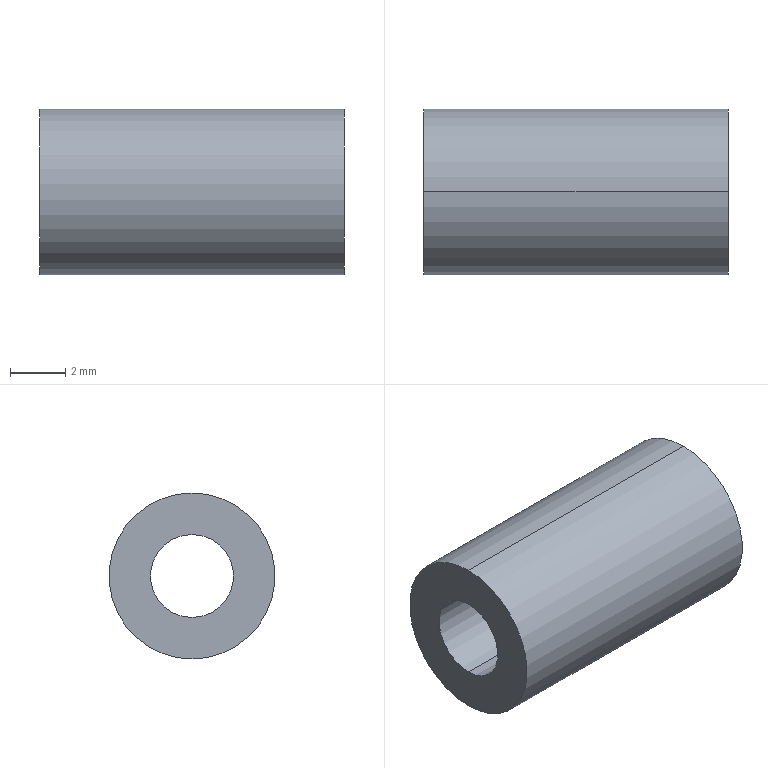Part | STEP file | Stud_1 | 1 solid | 6 faces | box 11 x 6 x 6 mm | volume 233.263 mm3 | cylinder 4 | plane 2 | commonest cylinder face diameters 3 x2 6 x2
STEP:
#1=CARTESIAN_POINT('',(0.,0.,0.));
#2=DIRECTION('',(0.,0.,1.));
#3=DIRECTION('',(1.,0.,0.));
#4=AXIS2_PLACEMENT_3D('',#1,#2,#3);
#5=CARTESIAN_POINT('',(11.,0.,3.));
#6=VERTEX_POINT('',#5);
#7=CARTESIAN_POINT('',(11.,0.,-3.));
#8=VERTEX_POINT('',#7);
#9=CARTESIAN_POINT('',(11.,0.,0.));
#10=DIRECTION('',(-1.,0.,0.));
#11=DIRECTION('',(0.,0.,1.));
#12=AXIS2_PLACEMENT_3D('',#9,#10,#11);
#13=CIRCLE('',#12,3.);
#14=CARTESIAN_POINT('',(11.,0.,0.));
#15=DIRECTION('',(-1.,0.,0.));
#16=DIRECTION('',(0.,0.,1.));
#17=AXIS2_PLACEMENT_3D('',#14,#15,#16);
#18=CYLINDRICAL_SURFACE('',#17,3.);
#19=CARTESIAN_POINT('',(0.,0.));
#20=DIRECTION('',(1.,0.));
#21=VECTOR('',#20,1.);
#22=LINE('',#19,#21);
#23=(GEOMETRIC_REPRESENTATION_CONTEXT(2)PARAMETRIC_REPRESENTATION_CONTEXT()REPRESENTATION_CONTEXT('',''));
#24=DEFINITIONAL_REPRESENTATION('',(#22),#23);
#25=PCURVE('',#18,#24);
#26=CARTESIAN_POINT('',(11.,0.,0.));
#27=DIRECTION('',(1.,0.,0.));
#28=DIRECTION('',(0.,0.,-1.));
#29=AXIS2_PLACEMENT_3D('',#26,#27,#28);
#30=PLANE('',#29);
#31=CARTESIAN_POINT('',(-3.,0.));
#32=CARTESIAN_POINT('',(-3.,5.196));
#33=CARTESIAN_POINT('',(1.5,2.598));
#34=CARTESIAN_POINT('',(6.,0.));
#35=CARTESIAN_POINT('',(1.5,-2.598));
#36=CARTESIAN_POINT('',(-3.,-5.196));
#37=CARTESIAN_POINT('',(-3.,0.));
#38=(BOUNDED_CURVE()B_SPLINE_CURVE(2,(#31,#32,#33,#34,#35,#36,#37),.UNSPECIFIED.,.T.,.F.)B_SPLINE_CURVE_WITH_KNOTS((1,2,2,2,2,1),(-2.094,0.,2.094,4.189,6.283,8.378),.UNSPECIFIED.)CURVE()GEOMETRIC_REPRESENTATION_ITEM()RATIONAL_B_SPLINE_CURVE((1.,0.5,1.,0.5,1.,0.5,1.))REPRESENTATION_ITEM(''));
#39=(GEOMETRIC_REPRESENTATION_CONTEXT(2)PARAMETRIC_REPRESENTATION_CONTEXT()REPRESENTATION_CONTEXT('',''));
#40=DEFINITIONAL_REPRESENTATION('',(#38),#39);
#41=PCURVE('',#30,#40);
#42=SURFACE_CURVE('',#13,(#25,#41),.PCURVE_S1.);
#43=EDGE_CURVE('',#6,#8,#42,.T.);
#44=ORIENTED_EDGE('',*,*,#43,.T.);
#45=CARTESIAN_POINT('',(0.,0.,-3.));
#46=VERTEX_POINT('',#45);
#47=CARTESIAN_POINT('',(11.,0.,-3.));
#48=DIRECTION('',(-1.,0.,0.));
#49=VECTOR('',#48,1.);
#50=LINE('',#47,#49);
#51=CARTESIAN_POINT('',(3.142,0.));
#52=DIRECTION('',(0.,1.));
#53=VECTOR('',#52,1.);
#54=LINE('',#51,#53);
#55=(GEOMETRIC_REPRESENTATION_CONTEXT(2)PARAMETRIC_REPRESENTATION_CONTEXT()REPRESENTATION_CONTEXT('',''));
#56=DEFINITIONAL_REPRESENTATION('',(#54),#55);
#57=PCURVE('',#18,#56);
#58=CARTESIAN_POINT('',(11.,0.,0.));
#59=DIRECTION('',(-1.,0.,0.));
#60=DIRECTION('',(0.,0.,1.));
#61=AXIS2_PLACEMENT_3D('',#58,#59,#60);
#62=CYLINDRICAL_SURFACE('',#61,3.);
#63=CARTESIAN_POINT('',(3.142,0.));
#64=DIRECTION('',(0.,1.));
#65=VECTOR('',#64,1.);
#66=LINE('',#63,#65);
#67=(GEOMETRIC_REPRESENTATION_CONTEXT(2)PARAMETRIC_REPRESENTATION_CONTEXT()REPRESENTATION_CONTEXT('',''));
#68=DEFINITIONAL_REPRESENTATION('',(#66),#67);
#69=PCURVE('',#62,#68);
#70=SURFACE_CURVE('',#50,(#57,#69),.PCURVE_S1.);
#71=EDGE_CURVE('',#8,#46,#70,.T.);
#72=ORIENTED_EDGE('',*,*,#71,.T.);
#73=CARTESIAN_POINT('',(0.,0.,3.));
#74=VERTEX_POINT('',#73);
#75=CARTESIAN_POINT('',(0.,0.,0.));
#76=DIRECTION('',(1.,0.,0.));
#77=DIRECTION('',(0.,0.,1.));
#78=AXIS2_PLACEMENT_3D('',#75,#76,#77);
#79=CIRCLE('',#78,3.);
#80=CARTESIAN_POINT('',(6.283,11.));
#81=DIRECTION('',(-1.,0.));
#82=VECTOR('',#81,1.);
#83=LINE('',#80,#82);
#84=(GEOMETRIC_REPRESENTATION_CONTEXT(2)PARAMETRIC_REPRESENTATION_CONTEXT()REPRESENTATION_CONTEXT('',''));
#85=DEFINITIONAL_REPRESENTATION('',(#83),#84);
#86=PCURVE('',#18,#85);
#87=CARTESIAN_POINT('',(0.,0.,0.));
#88=DIRECTION('',(1.,0.,0.));
#89=DIRECTION('',(0.,0.,-1.));
#90=AXIS2_PLACEMENT_3D('',#87,#88,#89);
#91=PLANE('',#90);
#92=CARTESIAN_POINT('',(0.,0.));
#93=DIRECTION('',(-1.,0.));
#94=AXIS2_PLACEMENT_2D('',#92,#93);
#95=CIRCLE('',#94,3.);
#96=(GEOMETRIC_REPRESENTATION_CONTEXT(2)PARAMETRIC_REPRESENTATION_CONTEXT()REPRESENTATION_CONTEXT('',''));
#97=DEFINITIONAL_REPRESENTATION('',(#95),#96);
#98=PCURVE('',#91,#97);
#99=SURFACE_CURVE('',#79,(#86,#98),.PCURVE_S1.);
#100=EDGE_CURVE('',#46,#74,#99,.T.);
#101=ORIENTED_EDGE('',*,*,#100,.T.);
#102=CARTESIAN_POINT('',(11.,0.,3.));
#103=DIRECTION('',(-1.,0.,0.));
#104=VECTOR('',#103,1.);
#105=LINE('',#102,#104);
#106=CARTESIAN_POINT('',(0.,0.));
#107=DIRECTION('',(0.,1.));
#108=VECTOR('',#107,1.);
#109=LINE('',#106,#108);
#110=(GEOMETRIC_REPRESENTATION_CONTEXT(2)PARAMETRIC_REPRESENTATION_CONTEXT()REPRESENTATION_CONTEXT('',''));
#111=DEFINITIONAL_REPRESENTATION('',(#109),#110);
#112=PCURVE('',#18,#111);
#113=CARTESIAN_POINT('',(6.283,0.));
#114=DIRECTION('',(0.,1.));
#115=VECTOR('',#114,1.);
#116=LINE('',#113,#115);
#117=(GEOMETRIC_REPRESENTATION_CONTEXT(2)PARAMETRIC_REPRESENTATION_CONTEXT()REPRESENTATION_CONTEXT('',''));
#118=DEFINITIONAL_REPRESENTATION('',(#116),#117);
#119=PCURVE('',#62,#118);
#120=SURFACE_CURVE('',#105,(#112,#119),.PCURVE_S1.);
#121=EDGE_CURVE('',#6,#74,#120,.T.);
#122=ORIENTED_EDGE('',*,*,#121,.F.);
#123=EDGE_LOOP('',(#44,#72,#101,#122));
#124=FACE_BOUND('',#123,.T.);
#125=ADVANCED_FACE('',(#124),#18,.T.);
#126=CARTESIAN_POINT('',(11.,0.,1.5));
#127=VERTEX_POINT('',#126);
#128=CARTESIAN_POINT('',(0.,0.,1.5));
#129=VERTEX_POINT('',#128);
#130=CARTESIAN_POINT('',(11.,0.,1.5));
#131=DIRECTION('',(-1.,0.,0.));
#132=VECTOR('',#131,1.);
#133=LINE('',#130,#132);
#134=CARTESIAN_POINT('',(11.,0.,0.));
#135=DIRECTION('',(-1.,0.,0.));
#136=DIRECTION('',(0.,0.,1.));
#137=AXIS2_PLACEMENT_3D('',#134,#135,#136);
#138=CYLINDRICAL_SURFACE('',#137,1.5);
#139=CARTESIAN_POINT('',(6.283,0.));
#140=DIRECTION('',(0.,1.));
#141=VECTOR('',#140,1.);
#142=LINE('',#139,#141);
#143=(GEOMETRIC_REPRESENTATION_CONTEXT(2)PARAMETRIC_REPRESENTATION_CONTEXT()REPRESENTATION_CONTEXT('',''));
#144=DEFINITIONAL_REPRESENTATION('',(#142),#143);
#145=PCURVE('',#138,#144);
#146=CARTESIAN_POINT('',(11.,0.,0.));
#147=DIRECTION('',(-1.,0.,0.));
#148=DIRECTION('',(0.,0.,1.));
#149=AXIS2_PLACEMENT_3D('',#146,#147,#148);
#150=CYLINDRICAL_SURFACE('',#149,1.5);
#151=CARTESIAN_POINT('',(0.,0.));
#152=DIRECTION('',(0.,1.));
#153=VECTOR('',#152,1.);
#154=LINE('',#151,#153);
#155=(GEOMETRIC_REPRESENTATION_CONTEXT(2)PARAMETRIC_REPRESENTATION_CONTEXT()REPRESENTATION_CONTEXT('',''));
#156=DEFINITIONAL_REPRESENTATION('',(#154),#155);
#157=PCURVE('',#150,#156);
#158=SURFACE_CURVE('',#133,(#145,#157),.PCURVE_S1.);
#159=EDGE_CURVE('',#127,#129,#158,.T.);
#160=ORIENTED_EDGE('',*,*,#159,.T.);
#161=CARTESIAN_POINT('',(0.,0.,-1.5));
#162=VERTEX_POINT('',#161);
#163=CARTESIAN_POINT('',(0.,0.,0.));
#164=DIRECTION('',(-1.,0.,0.));
#165=DIRECTION('',(0.,0.,1.));
#166=AXIS2_PLACEMENT_3D('',#163,#164,#165);
#167=CIRCLE('',#166,1.5);
#168=CARTESIAN_POINT('',(0.,11.));
#169=DIRECTION('',(1.,0.));
#170=VECTOR('',#169,1.);
#171=LINE('',#168,#170);
#172=(GEOMETRIC_REPRESENTATION_CONTEXT(2)PARAMETRIC_REPRESENTATION_CONTEXT()REPRESENTATION_CONTEXT('',''));
#173=DEFINITIONAL_REPRESENTATION('',(#171),#172);
#174=PCURVE('',#138,#173);
#175=CARTESIAN_POINT('',(-1.5,0.));
#176=CARTESIAN_POINT('',(-1.5,2.598));
#177=CARTESIAN_POINT('',(0.75,1.299));
#178=CARTESIAN_POINT('',(3.,0.));
#179=CARTESIAN_POINT('',(0.75,-1.299));
#180=CARTESIAN_POINT('',(-1.5,-2.598));
#181=CARTESIAN_POINT('',(-1.5,0.));
#182=(BOUNDED_CURVE()B_SPLINE_CURVE(2,(#175,#176,#177,#178,#179,#180,#181),.UNSPECIFIED.,.T.,.F.)B_SPLINE_CURVE_WITH_KNOTS((1,2,2,2,2,1),(-2.094,0.,2.094,4.189,6.283,8.378),.UNSPECIFIED.)CURVE()GEOMETRIC_REPRESENTATION_ITEM()RATIONAL_B_SPLINE_CURVE((1.,0.5,1.,0.5,1.,0.5,1.))REPRESENTATION_ITEM(''));
#183=(GEOMETRIC_REPRESENTATION_CONTEXT(2)PARAMETRIC_REPRESENTATION_CONTEXT()REPRESENTATION_CONTEXT('',''));
#184=DEFINITIONAL_REPRESENTATION('',(#182),#183);
#185=PCURVE('',#91,#184);
#186=SURFACE_CURVE('',#167,(#174,#185),.PCURVE_S1.);
#187=EDGE_CURVE('',#162,#129,#186,.T.);
#188=ORIENTED_EDGE('',*,*,#187,.F.);
#189=CARTESIAN_POINT('',(11.,0.,-1.5));
#190=VERTEX_POINT('',#189);
#191=CARTESIAN_POINT('',(11.,0.,-1.5));
#192=DIRECTION('',(-1.,0.,0.));
#193=VECTOR('',#192,1.);
#194=LINE('',#191,#193);
#195=CARTESIAN_POINT('',(3.142,0.));
#196=DIRECTION('',(0.,1.));
#197=VECTOR('',#196,1.);
#198=LINE('',#195,#197);
#199=(GEOMETRIC_REPRESENTATION_CONTEXT(2)PARAMETRIC_REPRESENTATION_CONTEXT()REPRESENTATION_CONTEXT('',''));
#200=DEFINITIONAL_REPRESENTATION('',(#198),#199);
#201=PCURVE('',#138,#200);
#202=CARTESIAN_POINT('',(3.142,0.));
#203=DIRECTION('',(0.,1.));
#204=VECTOR('',#203,1.);
#205=LINE('',#202,#204);
#206=(GEOMETRIC_REPRESENTATION_CONTEXT(2)PARAMETRIC_REPRESENTATION_CONTEXT()REPRESENTATION_CONTEXT('',''));
#207=DEFINITIONAL_REPRESENTATION('',(#205),#206);
#208=PCURVE('',#150,#207);
#209=SURFACE_CURVE('',#194,(#201,#208),.PCURVE_S1.);
#210=EDGE_CURVE('',#190,#162,#209,.T.);
#211=ORIENTED_EDGE('',*,*,#210,.F.);
#212=CARTESIAN_POINT('',(11.,0.,0.));
#213=DIRECTION('',(-1.,0.,0.));
#214=DIRECTION('',(0.,0.,1.));
#215=AXIS2_PLACEMENT_3D('',#212,#213,#214);
#216=CIRCLE('',#215,1.5);
#217=CARTESIAN_POINT('',(0.,0.));
#218=DIRECTION('',(1.,0.));
#219=VECTOR('',#218,1.);
#220=LINE('',#217,#219);
#221=(GEOMETRIC_REPRESENTATION_CONTEXT(2)PARAMETRIC_REPRESENTATION_CONTEXT()REPRESENTATION_CONTEXT('',''));
#222=DEFINITIONAL_REPRESENTATION('',(#220),#221);
#223=PCURVE('',#138,#222);
#224=CARTESIAN_POINT('',(-1.5,0.));
#225=CARTESIAN_POINT('',(-1.5,2.598));
#226=CARTESIAN_POINT('',(0.75,1.299));
#227=CARTESIAN_POINT('',(3.,0.));
#228=CARTESIAN_POINT('',(0.75,-1.299));
#229=CARTESIAN_POINT('',(-1.5,-2.598));
#230=CARTESIAN_POINT('',(-1.5,0.));
#231=(BOUNDED_CURVE()B_SPLINE_CURVE(2,(#224,#225,#226,#227,#228,#229,#230),.UNSPECIFIED.,.T.,.F.)B_SPLINE_CURVE_WITH_KNOTS((1,2,2,2,2,1),(-2.094,0.,2.094,4.189,6.283,8.378),.UNSPECIFIED.)CURVE()GEOMETRIC_REPRESENTATION_ITEM()RATIONAL_B_SPLINE_CURVE((1.,0.5,1.,0.5,1.,0.5,1.))REPRESENTATION_ITEM(''));
#232=(GEOMETRIC_REPRESENTATION_CONTEXT(2)PARAMETRIC_REPRESENTATION_CONTEXT()REPRESENTATION_CONTEXT('',''));
#233=DEFINITIONAL_REPRESENTATION('',(#231),#232);
#234=PCURVE('',#30,#233);
#235=SURFACE_CURVE('',#216,(#223,#234),.PCURVE_S1.);
#236=EDGE_CURVE('',#190,#127,#235,.T.);
#237=ORIENTED_EDGE('',*,*,#236,.T.);
#238=EDGE_LOOP('',(#160,#188,#211,#237));
#239=FACE_BOUND('',#238,.F.);
#240=ADVANCED_FACE('',(#239),#138,.F.);
#241=ORIENTED_EDGE('',*,*,#71,.F.);
#242=CARTESIAN_POINT('',(11.,0.,0.));
#243=DIRECTION('',(-1.,0.,0.));
#244=DIRECTION('',(0.,0.,1.));
#245=AXIS2_PLACEMENT_3D('',#242,#243,#244);
#246=CIRCLE('',#245,3.);
#247=CARTESIAN_POINT('',(0.,0.));
#248=DIRECTION('',(1.,0.));
#249=VECTOR('',#248,1.);
#250=LINE('',#247,#249);
#251=(GEOMETRIC_REPRESENTATION_CONTEXT(2)PARAMETRIC_REPRESENTATION_CONTEXT()REPRESENTATION_CONTEXT('',''));
#252=DEFINITIONAL_REPRESENTATION('',(#250),#251);
#253=PCURVE('',#62,#252);
#254=CARTESIAN_POINT('',(-3.,0.));
#255=CARTESIAN_POINT('',(-3.,5.196));
#256=CARTESIAN_POINT('',(1.5,2.598));
#257=CARTESIAN_POINT('',(6.,0.));
#258=CARTESIAN_POINT('',(1.5,-2.598));
#259=CARTESIAN_POINT('',(-3.,-5.196));
#260=CARTESIAN_POINT('',(-3.,0.));
#261=(BOUNDED_CURVE()B_SPLINE_CURVE(2,(#254,#255,#256,#257,#258,#259,#260),.UNSPECIFIED.,.T.,.F.)B_SPLINE_CURVE_WITH_KNOTS((1,2,2,2,2,1),(-2.094,0.,2.094,4.189,6.283,8.378),.UNSPECIFIED.)CURVE()GEOMETRIC_REPRESENTATION_ITEM()RATIONAL_B_SPLINE_CURVE((1.,0.5,1.,0.5,1.,0.5,1.))REPRESENTATION_ITEM(''));
#262=(GEOMETRIC_REPRESENTATION_CONTEXT(2)PARAMETRIC_REPRESENTATION_CONTEXT()REPRESENTATION_CONTEXT('',''));
#263=DEFINITIONAL_REPRESENTATION('',(#261),#262);
#264=PCURVE('',#30,#263);
#265=SURFACE_CURVE('',#246,(#253,#264),.PCURVE_S1.);
#266=EDGE_CURVE('',#8,#6,#265,.T.);
#267=ORIENTED_EDGE('',*,*,#266,.T.);
#268=ORIENTED_EDGE('',*,*,#121,.T.);
#269=CARTESIAN_POINT('',(0.,0.,0.));
#270=DIRECTION('',(1.,0.,0.));
#271=DIRECTION('',(0.,0.,1.));
#272=AXIS2_PLACEMENT_3D('',#269,#270,#271);
#273=CIRCLE('',#272,3.);
#274=CARTESIAN_POINT('',(6.283,11.));
#275=DIRECTION('',(-1.,0.));
#276=VECTOR('',#275,1.);
#277=LINE('',#274,#276);
#278=(GEOMETRIC_REPRESENTATION_CONTEXT(2)PARAMETRIC_REPRESENTATION_CONTEXT()REPRESENTATION_CONTEXT('',''));
#279=DEFINITIONAL_REPRESENTATION('',(#277),#278);
#280=PCURVE('',#62,#279);
#281=CARTESIAN_POINT('',(0.,0.));
#282=DIRECTION('',(-1.,0.));
#283=AXIS2_PLACEMENT_2D('',#281,#282);
#284=CIRCLE('',#283,3.);
#285=(GEOMETRIC_REPRESENTATION_CONTEXT(2)PARAMETRIC_REPRESENTATION_CONTEXT()REPRESENTATION_CONTEXT('',''));
#286=DEFINITIONAL_REPRESENTATION('',(#284),#285);
#287=PCURVE('',#91,#286);
#288=SURFACE_CURVE('',#273,(#280,#287),.PCURVE_S1.);
#289=EDGE_CURVE('',#74,#46,#288,.T.);
#290=ORIENTED_EDGE('',*,*,#289,.T.);
#291=EDGE_LOOP('',(#241,#267,#268,#290));
#292=FACE_BOUND('',#291,.T.);
#293=ADVANCED_FACE('',(#292),#62,.T.);
#294=CARTESIAN_POINT('',(0.,0.,0.));
#295=DIRECTION('',(-1.,0.,0.));
#296=DIRECTION('',(0.,0.,1.));
#297=AXIS2_PLACEMENT_3D('',#294,#295,#296);
#298=CIRCLE('',#297,1.5);
#299=CARTESIAN_POINT('',(-1.5,0.));
#300=CARTESIAN_POINT('',(-1.5,2.598));
#301=CARTESIAN_POINT('',(0.75,1.299));
#302=CARTESIAN_POINT('',(3.,0.));
#303=CARTESIAN_POINT('',(0.75,-1.299));
#304=CARTESIAN_POINT('',(-1.5,-2.598));
#305=CARTESIAN_POINT('',(-1.5,0.));
#306=(BOUNDED_CURVE()B_SPLINE_CURVE(2,(#299,#300,#301,#302,#303,#304,#305),.UNSPECIFIED.,.T.,.F.)B_SPLINE_CURVE_WITH_KNOTS((1,2,2,2,2,1),(-2.094,0.,2.094,4.189,6.283,8.378),.UNSPECIFIED.)CURVE()GEOMETRIC_REPRESENTATION_ITEM()RATIONAL_B_SPLINE_CURVE((1.,0.5,1.,0.5,1.,0.5,1.))REPRESENTATION_ITEM(''));
#307=(GEOMETRIC_REPRESENTATION_CONTEXT(2)PARAMETRIC_REPRESENTATION_CONTEXT()REPRESENTATION_CONTEXT('',''));
#308=DEFINITIONAL_REPRESENTATION('',(#306),#307);
#309=PCURVE('',#91,#308);
#310=CARTESIAN_POINT('',(0.,11.));
#311=DIRECTION('',(1.,0.));
#312=VECTOR('',#311,1.);
#313=LINE('',#310,#312);
#314=(GEOMETRIC_REPRESENTATION_CONTEXT(2)PARAMETRIC_REPRESENTATION_CONTEXT()REPRESENTATION_CONTEXT('',''));
#315=DEFINITIONAL_REPRESENTATION('',(#313),#314);
#316=PCURVE('',#150,#315);
#317=SURFACE_CURVE('',#298,(#309,#316),.PCURVE_S1.);
#318=EDGE_CURVE('',#129,#162,#317,.T.);
#319=ORIENTED_EDGE('',*,*,#318,.F.);
#320=ORIENTED_EDGE('',*,*,#187,.F.);
#321=EDGE_LOOP('',(#319,#320));
#322=FACE_BOUND('',#321,.T.);
#323=ORIENTED_EDGE('',*,*,#289,.F.);
#324=ORIENTED_EDGE('',*,*,#100,.F.);
#325=EDGE_LOOP('',(#323,#324));
#326=FACE_BOUND('',#325,.T.);
#327=ADVANCED_FACE('',(#322,#326),#91,.F.);
#328=CARTESIAN_POINT('',(11.,0.,0.));
#329=DIRECTION('',(-1.,0.,0.));
#330=DIRECTION('',(0.,0.,1.));
#331=AXIS2_PLACEMENT_3D('',#328,#329,#330);
#332=CIRCLE('',#331,1.5);
#333=CARTESIAN_POINT('',(-1.5,0.));
#334=CARTESIAN_POINT('',(-1.5,2.598));
#335=CARTESIAN_POINT('',(0.75,1.299));
#336=CARTESIAN_POINT('',(3.,0.));
#337=CARTESIAN_POINT('',(0.75,-1.299));
#338=CARTESIAN_POINT('',(-1.5,-2.598));
#339=CARTESIAN_POINT('',(-1.5,0.));
#340=(BOUNDED_CURVE()B_SPLINE_CURVE(2,(#333,#334,#335,#336,#337,#338,#339),.UNSPECIFIED.,.T.,.F.)B_SPLINE_CURVE_WITH_KNOTS((1,2,2,2,2,1),(-2.094,0.,2.094,4.189,6.283,8.378),.UNSPECIFIED.)CURVE()GEOMETRIC_REPRESENTATION_ITEM()RATIONAL_B_SPLINE_CURVE((1.,0.5,1.,0.5,1.,0.5,1.))REPRESENTATION_ITEM(''));
#341=(GEOMETRIC_REPRESENTATION_CONTEXT(2)PARAMETRIC_REPRESENTATION_CONTEXT()REPRESENTATION_CONTEXT('',''));
#342=DEFINITIONAL_REPRESENTATION('',(#340),#341);
#343=PCURVE('',#30,#342);
#344=CARTESIAN_POINT('',(0.,0.));
#345=DIRECTION('',(1.,0.));
#346=VECTOR('',#345,1.);
#347=LINE('',#344,#346);
#348=(GEOMETRIC_REPRESENTATION_CONTEXT(2)PARAMETRIC_REPRESENTATION_CONTEXT()REPRESENTATION_CONTEXT('',''));
#349=DEFINITIONAL_REPRESENTATION('',(#347),#348);
#350=PCURVE('',#150,#349);
#351=SURFACE_CURVE('',#332,(#343,#350),.PCURVE_S1.);
#352=EDGE_CURVE('',#127,#190,#351,.T.);
#353=ORIENTED_EDGE('',*,*,#352,.T.);
#354=ORIENTED_EDGE('',*,*,#236,.T.);
#355=EDGE_LOOP('',(#353,#354));
#356=FACE_BOUND('',#355,.T.);
#357=ORIENTED_EDGE('',*,*,#43,.F.);
#358=ORIENTED_EDGE('',*,*,#266,.F.);
#359=EDGE_LOOP('',(#357,#358));
#360=FACE_BOUND('',#359,.T.);
#361=ADVANCED_FACE('',(#356,#360),#30,.T.);
#362=ORIENTED_EDGE('',*,*,#318,.F.);
#363=ORIENTED_EDGE('',*,*,#159,.F.);
#364=ORIENTED_EDGE('',*,*,#352,.T.);
#365=ORIENTED_EDGE('',*,*,#210,.T.);
#366=EDGE_LOOP('',(#362,#363,#364,#365));
#367=FACE_BOUND('',#366,.F.);
#368=ADVANCED_FACE('',(#367),#150,.F.);
#369=CLOSED_SHELL('',(#125,#240,#293,#327,#361,#368));
#370=MANIFOLD_SOLID_BREP('',#369);
#371=(LENGTH_UNIT()NAMED_UNIT(*)SI_UNIT(.MILLI.,.METRE.));
#372=UNCERTAINTY_MEASURE_WITH_UNIT(LENGTH_MEASURE(0.0000001),#371,'','');
#373=(NAMED_UNIT(*)PLANE_ANGLE_UNIT()SI_UNIT($,.RADIAN.));
#374=(NAMED_UNIT(*)SI_UNIT($,.STERADIAN.)SOLID_ANGLE_UNIT());
#375=(GEOMETRIC_REPRESENTATION_CONTEXT(3)GLOBAL_UNCERTAINTY_ASSIGNED_CONTEXT((#372))GLOBAL_UNIT_ASSIGNED_CONTEXT((#371,#373,#374))REPRESENTATION_CONTEXT('',''));
#376=ADVANCED_BREP_SHAPE_REPRESENTATION('',(#4,#370),#375);